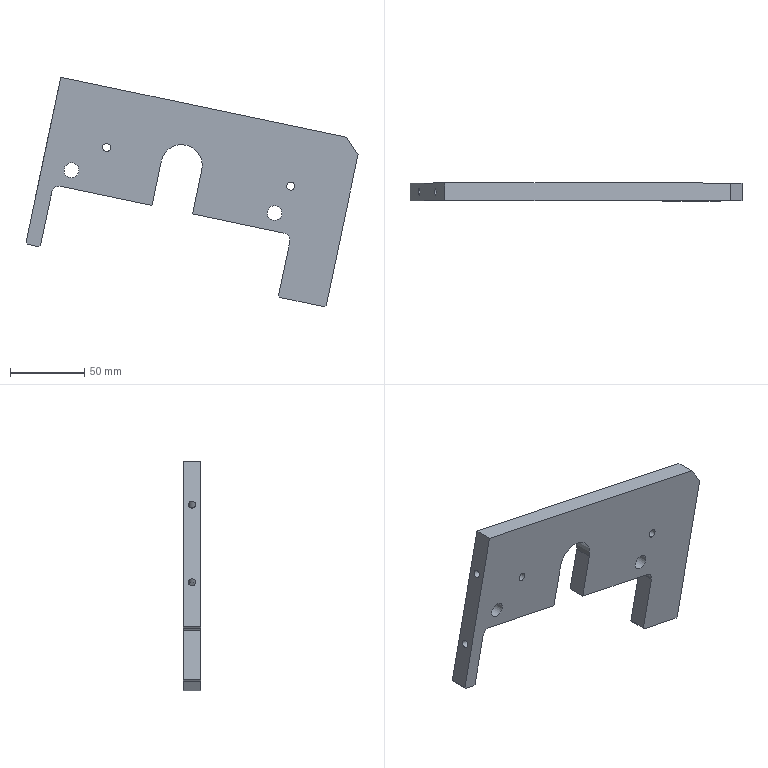Part | STEP file | BERCO_004 | 1 solid | 32 faces | box 223.963 x 12 x 154.905 mm | volume 182941 mm3 | plane 20 | cylinder 11 | cone 1 | commonest cylinder face diameters 10 x3 4.917 x2 5.5 x2 9 x2 10.1 x1 28 x1